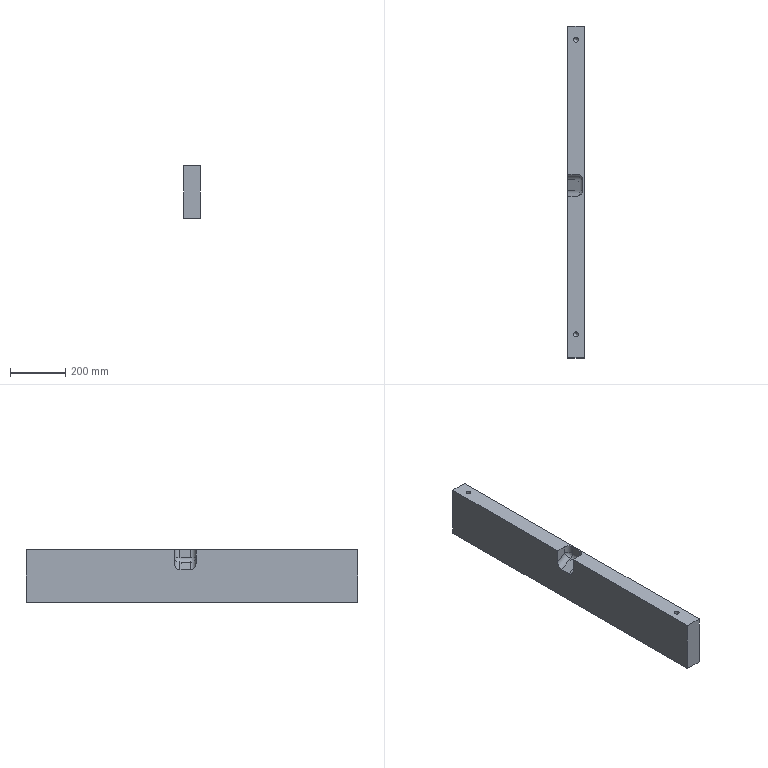Part | STEP file | lll_id4466_x_t | 1 solid | 26 faces | box 60 x 1200 x 190 mm | volume 13409835 mm3 | plane 10 | cylinder 9 | cone 5 | sphere 2 | commonest cylinder face diameters 40 x5 17.505 x2 17.506 x2
STEP:
#1=CARTESIAN_POINT('',(1461.188,550.,-370.));
#2=VERTEX_POINT('',#1);
#3=CARTESIAN_POINT('',(1452.435,550.,-370.));
#4=DIRECTION('',(0.,0.,1.));
#5=DIRECTION('',(1.,0.,0.));
#6=AXIS2_PLACEMENT_3D('',#3,#4,#5);
#7=CIRCLE('',#6,8.752);
#8=EDGE_CURVE('',#2,#2,#7,.T.);
#9=ORIENTED_EDGE('',*,*,#8,.T.);
#10=EDGE_LOOP('',(#9));
#11=FACE_BOUND('',#10,.T.);
#12=CARTESIAN_POINT('',(1422.435,600.,-370.));
#13=VERTEX_POINT('',#12);
#14=CARTESIAN_POINT('',(1422.435,-600.,-370.));
#15=VERTEX_POINT('',#14);
#16=CARTESIAN_POINT('',(1422.435,1.,-370.));
#17=DIRECTION('',(0.,-1.,0.));
#18=VECTOR('',#17,1.);
#19=LINE('',#16,#18);
#20=EDGE_CURVE('',#13,#15,#19,.T.);
#21=ORIENTED_EDGE('',*,*,#20,.F.);
#22=CARTESIAN_POINT('',(1482.435,600.,-370.));
#23=VERTEX_POINT('',#22);
#24=CARTESIAN_POINT('',(-2487.565,600.,-370.));
#25=DIRECTION('',(1.,0.,0.));
#26=VECTOR('',#25,1.);
#27=LINE('',#24,#26);
#28=EDGE_CURVE('',#13,#23,#27,.T.);
#29=ORIENTED_EDGE('',*,*,#28,.T.);
#30=CARTESIAN_POINT('',(1482.435,-600.,-370.));
#31=VERTEX_POINT('',#30);
#32=CARTESIAN_POINT('',(1482.435,600.,-370.));
#33=DIRECTION('',(0.,-1.,0.));
#34=VECTOR('',#33,1.);
#35=LINE('',#32,#34);
#36=EDGE_CURVE('',#23,#31,#35,.T.);
#37=ORIENTED_EDGE('',*,*,#36,.T.);
#38=CARTESIAN_POINT('',(1482.435,-600.,-370.));
#39=DIRECTION('',(-1.,0.,0.));
#40=VECTOR('',#39,1.);
#41=LINE('',#38,#40);
#42=EDGE_CURVE('',#31,#15,#41,.T.);
#43=ORIENTED_EDGE('',*,*,#42,.T.);
#44=EDGE_LOOP('',(#21,#29,#37,#43));
#45=FACE_BOUND('',#44,.T.);
#46=CARTESIAN_POINT('',(1461.188,-515.,-370.));
#47=VERTEX_POINT('',#46);
#48=CARTESIAN_POINT('',(1452.435,-515.,-370.));
#49=DIRECTION('',(0.,0.,1.));
#50=DIRECTION('',(1.,0.,0.));
#51=AXIS2_PLACEMENT_3D('',#48,#49,#50);
#52=CIRCLE('',#51,8.752);
#53=EDGE_CURVE('',#47,#47,#52,.T.);
#54=ORIENTED_EDGE('',*,*,#53,.T.);
#55=EDGE_LOOP('',(#54));
#56=FACE_BOUND('',#55,.T.);
#57=CARTESIAN_POINT('',(3668.751,1.,-370.));
#58=DIRECTION('',(0.,0.,-1.));
#59=DIRECTION('',(-1.,0.,0.));
#60=AXIS2_PLACEMENT_3D('',#57,#58,#59);
#61=PLANE('',#60);
#62=ADVANCED_FACE('',(#11,#45,#56),#61,.T.);
#63=CARTESIAN_POINT('',(1422.435,-15.,-180.));
#64=VERTEX_POINT('',#63);
#65=CARTESIAN_POINT('',(1422.435,-15.,-229.633));
#66=VERTEX_POINT('',#65);
#67=CARTESIAN_POINT('',(1422.435,-15.,-251.25));
#68=DIRECTION('',(0.,0.,-1.));
#69=VECTOR('',#68,1.);
#70=LINE('',#67,#69);
#71=EDGE_CURVE('',#64,#66,#70,.T.);
#72=ORIENTED_EDGE('',*,*,#71,.T.);
#73=CARTESIAN_POINT('',(1422.435,5.,-252.727));
#74=VERTEX_POINT('',#73);
#75=CARTESIAN_POINT('',(1422.435,5.,-229.633));
#76=DIRECTION('',(1.,0.,0.));
#77=DIRECTION('',(0.,0.,1.));
#78=AXIS2_PLACEMENT_3D('',#75,#76,#77);
#79=ELLIPSE('',#78,23.094,20.);
#80=EDGE_CURVE('',#66,#74,#79,.T.);
#81=ORIENTED_EDGE('',*,*,#80,.T.);
#82=CARTESIAN_POINT('',(1422.435,43.5,-252.727));
#83=VERTEX_POINT('',#82);
#84=CARTESIAN_POINT('',(1422.435,0.,-252.727));
#85=DIRECTION('',(0.,1.,0.));
#86=VECTOR('',#85,1.);
#87=LINE('',#84,#86);
#88=EDGE_CURVE('',#74,#83,#87,.T.);
#89=ORIENTED_EDGE('',*,*,#88,.T.);
#90=CARTESIAN_POINT('',(1422.435,63.5,-229.633));
#91=VERTEX_POINT('',#90);
#92=CARTESIAN_POINT('',(1422.435,43.5,-229.633));
#93=DIRECTION('',(1.,0.,0.));
#94=DIRECTION('',(0.,0.,-1.));
#95=AXIS2_PLACEMENT_3D('',#92,#93,#94);
#96=ELLIPSE('',#95,23.094,20.);
#97=EDGE_CURVE('',#83,#91,#96,.T.);
#98=ORIENTED_EDGE('',*,*,#97,.T.);
#99=CARTESIAN_POINT('',(1422.435,63.5,-180.));
#100=VERTEX_POINT('',#99);
#101=CARTESIAN_POINT('',(1422.435,63.5,-251.25));
#102=DIRECTION('',(0.,0.,1.));
#103=VECTOR('',#102,1.);
#104=LINE('',#101,#103);
#105=EDGE_CURVE('',#91,#100,#104,.T.);
#106=ORIENTED_EDGE('',*,*,#105,.T.);
#107=CARTESIAN_POINT('',(1422.435,600.,-180.));
#108=VERTEX_POINT('',#107);
#109=CARTESIAN_POINT('',(1422.435,0.,-180.));
#110=DIRECTION('',(0.,1.,0.));
#111=VECTOR('',#110,1.);
#112=LINE('',#109,#111);
#113=EDGE_CURVE('',#100,#108,#112,.T.);
#114=ORIENTED_EDGE('',*,*,#113,.T.);
#115=CARTESIAN_POINT('',(1422.435,600.,-182.5));
#116=DIRECTION('',(0.,0.,1.));
#117=VECTOR('',#116,1.);
#118=LINE('',#115,#117);
#119=EDGE_CURVE('',#13,#108,#118,.T.);
#120=ORIENTED_EDGE('',*,*,#119,.F.);
#121=ORIENTED_EDGE('',*,*,#20,.T.);
#122=CARTESIAN_POINT('',(1422.435,-600.,-180.));
#123=VERTEX_POINT('',#122);
#124=CARTESIAN_POINT('',(1422.435,-600.,-182.5));
#125=DIRECTION('',(0.,0.,-1.));
#126=VECTOR('',#125,1.);
#127=LINE('',#124,#126);
#128=EDGE_CURVE('',#123,#15,#127,.T.);
#129=ORIENTED_EDGE('',*,*,#128,.F.);
#130=CARTESIAN_POINT('',(1422.435,0.,-180.));
#131=DIRECTION('',(0.,1.,0.));
#132=VECTOR('',#131,1.);
#133=LINE('',#130,#132);
#134=EDGE_CURVE('',#123,#64,#133,.T.);
#135=ORIENTED_EDGE('',*,*,#134,.T.);
#136=EDGE_LOOP('',(#72,#81,#89,#98,#106,#114,#120,#121,#129,#135));
#137=FACE_OUTER_BOUND('',#136,.T.);
#138=CARTESIAN_POINT('',(1422.435,0.,-251.25));
#139=DIRECTION('',(1.,0.,0.));
#140=DIRECTION('',(0.,0.,-1.));
#141=AXIS2_PLACEMENT_3D('',#138,#139,#140);
#142=PLANE('',#141);
#143=ADVANCED_FACE('',(#137),#142,.F.);
#144=ORIENTED_EDGE('',*,*,#36,.F.);
#145=CARTESIAN_POINT('',(1482.435,600.,-180.));
#146=VERTEX_POINT('',#145);
#147=CARTESIAN_POINT('',(1482.435,600.,-182.5));
#148=DIRECTION('',(0.,0.,-1.));
#149=VECTOR('',#148,1.);
#150=LINE('',#147,#149);
#151=EDGE_CURVE('',#146,#23,#150,.T.);
#152=ORIENTED_EDGE('',*,*,#151,.F.);
#153=CARTESIAN_POINT('',(1482.435,-600.,-180.));
#154=VERTEX_POINT('',#153);
#155=CARTESIAN_POINT('',(1482.435,1.,-180.));
#156=DIRECTION('',(0.,-1.,0.));
#157=VECTOR('',#156,1.);
#158=LINE('',#155,#157);
#159=EDGE_CURVE('',#146,#154,#158,.T.);
#160=ORIENTED_EDGE('',*,*,#159,.T.);
#161=CARTESIAN_POINT('',(1482.435,-600.,-182.5));
#162=DIRECTION('',(0.,0.,-1.));
#163=VECTOR('',#162,1.);
#164=LINE('',#161,#163);
#165=EDGE_CURVE('',#154,#31,#164,.T.);
#166=ORIENTED_EDGE('',*,*,#165,.T.);
#167=EDGE_LOOP('',(#144,#152,#160,#166));
#168=FACE_OUTER_BOUND('',#167,.T.);
#169=CARTESIAN_POINT('',(1482.435,600.,-182.5));
#170=DIRECTION('',(1.,0.,0.));
#171=DIRECTION('',(0.,0.,-1.));
#172=AXIS2_PLACEMENT_3D('',#169,#170,#171);
#173=PLANE('',#172);
#174=ADVANCED_FACE('',(#168),#173,.T.);
#175=ORIENTED_EDGE('',*,*,#128,.T.);
#176=ORIENTED_EDGE('',*,*,#42,.F.);
#177=ORIENTED_EDGE('',*,*,#165,.F.);
#178=CARTESIAN_POINT('',(3668.751,-600.,-180.));
#179=DIRECTION('',(-1.,0.,0.));
#180=VECTOR('',#179,1.);
#181=LINE('',#178,#180);
#182=EDGE_CURVE('',#154,#123,#181,.T.);
#183=ORIENTED_EDGE('',*,*,#182,.T.);
#184=EDGE_LOOP('',(#175,#176,#177,#183));
#185=FACE_OUTER_BOUND('',#184,.T.);
#186=CARTESIAN_POINT('',(1482.435,-600.,-182.5));
#187=DIRECTION('',(0.,-1.,0.));
#188=DIRECTION('',(0.,0.,-1.));
#189=AXIS2_PLACEMENT_3D('',#186,#187,#188);
#190=PLANE('',#189);
#191=ADVANCED_FACE('',(#185),#190,.T.);
#192=ORIENTED_EDGE('',*,*,#119,.T.);
#193=CARTESIAN_POINT('',(3668.751,600.,-180.));
#194=DIRECTION('',(1.,0.,0.));
#195=VECTOR('',#194,1.);
#196=LINE('',#193,#195);
#197=EDGE_CURVE('',#108,#146,#196,.T.);
#198=ORIENTED_EDGE('',*,*,#197,.T.);
#199=ORIENTED_EDGE('',*,*,#151,.T.);
#200=ORIENTED_EDGE('',*,*,#28,.F.);
#201=EDGE_LOOP('',(#192,#198,#199,#200));
#202=FACE_OUTER_BOUND('',#201,.T.);
#203=CARTESIAN_POINT('',(-2487.565,600.,-182.5));
#204=DIRECTION('',(0.,1.,0.));
#205=DIRECTION('',(0.,0.,1.));
#206=AXIS2_PLACEMENT_3D('',#203,#204,#205);
#207=PLANE('',#206);
#208=ADVANCED_FACE('',(#202),#207,.T.);
#209=CARTESIAN_POINT('',(1443.682,550.,-180.));
#210=VERTEX_POINT('',#209);
#211=CARTESIAN_POINT('',(1452.435,550.,-180.));
#212=DIRECTION('',(0.,0.,-1.));
#213=DIRECTION('',(-1.,0.,0.));
#214=AXIS2_PLACEMENT_3D('',#211,#212,#213);
#215=CIRCLE('',#214,8.753);
#216=EDGE_CURVE('',#210,#210,#215,.T.);
#217=ORIENTED_EDGE('',*,*,#216,.T.);
#218=EDGE_LOOP('',(#217));
#219=FACE_BOUND('',#218,.T.);
#220=CARTESIAN_POINT('',(1443.682,-515.,-180.));
#221=VERTEX_POINT('',#220);
#222=CARTESIAN_POINT('',(1452.435,-515.,-180.));
#223=DIRECTION('',(0.,0.,-1.));
#224=DIRECTION('',(-1.,0.,0.));
#225=AXIS2_PLACEMENT_3D('',#222,#223,#224);
#226=CIRCLE('',#225,8.753);
#227=EDGE_CURVE('',#221,#221,#226,.T.);
#228=ORIENTED_EDGE('',*,*,#227,.T.);
#229=EDGE_LOOP('',(#228));
#230=FACE_BOUND('',#229,.T.);
#231=CARTESIAN_POINT('',(1457.5,63.5,-180.));
#232=VERTEX_POINT('',#231);
#233=CARTESIAN_POINT('',(3668.751,63.5,-180.));
#234=DIRECTION('',(1.,0.,0.));
#235=VECTOR('',#234,1.);
#236=LINE('',#233,#235);
#237=EDGE_CURVE('',#100,#232,#236,.T.);
#238=ORIENTED_EDGE('',*,*,#237,.T.);
#239=CARTESIAN_POINT('',(1477.5,43.5,-180.));
#240=VERTEX_POINT('',#239);
#241=CARTESIAN_POINT('',(1457.5,43.5,-180.));
#242=DIRECTION('',(0.,0.,-1.));
#243=DIRECTION('',(-1.,0.,0.));
#244=AXIS2_PLACEMENT_3D('',#241,#242,#243);
#245=CIRCLE('',#244,20.);
#246=EDGE_CURVE('',#232,#240,#245,.T.);
#247=ORIENTED_EDGE('',*,*,#246,.T.);
#248=CARTESIAN_POINT('',(1477.5,5.,-180.));
#249=VERTEX_POINT('',#248);
#250=CARTESIAN_POINT('',(1477.5,1.,-180.));
#251=DIRECTION('',(0.,-1.,0.));
#252=VECTOR('',#251,1.);
#253=LINE('',#250,#252);
#254=EDGE_CURVE('',#240,#249,#253,.T.);
#255=ORIENTED_EDGE('',*,*,#254,.T.);
#256=CARTESIAN_POINT('',(1457.5,-15.,-180.));
#257=VERTEX_POINT('',#256);
#258=CARTESIAN_POINT('',(1457.5,5.,-180.));
#259=DIRECTION('',(0.,0.,-1.));
#260=DIRECTION('',(-1.,0.,0.));
#261=AXIS2_PLACEMENT_3D('',#258,#259,#260);
#262=CIRCLE('',#261,20.);
#263=EDGE_CURVE('',#249,#257,#262,.T.);
#264=ORIENTED_EDGE('',*,*,#263,.T.);
#265=CARTESIAN_POINT('',(3668.751,-15.,-180.));
#266=DIRECTION('',(-1.,0.,0.));
#267=VECTOR('',#266,1.);
#268=LINE('',#265,#267);
#269=EDGE_CURVE('',#257,#64,#268,.T.);
#270=ORIENTED_EDGE('',*,*,#269,.T.);
#271=ORIENTED_EDGE('',*,*,#134,.F.);
#272=ORIENTED_EDGE('',*,*,#182,.F.);
#273=ORIENTED_EDGE('',*,*,#159,.F.);
#274=ORIENTED_EDGE('',*,*,#197,.F.);
#275=ORIENTED_EDGE('',*,*,#113,.F.);
#276=EDGE_LOOP('',(#238,#247,#255,#264,#270,#271,#272,#273,#274,#275));
#277=FACE_BOUND('',#276,.T.);
#278=CARTESIAN_POINT('',(3668.751,1.,-180.));
#279=DIRECTION('',(0.,0.,-1.));
#280=DIRECTION('',(-1.,0.,0.));
#281=AXIS2_PLACEMENT_3D('',#278,#279,#280);
#282=PLANE('',#281);
#283=ADVANCED_FACE('',(#219,#230,#277),#282,.F.);
#284=CARTESIAN_POINT('',(1457.5,-15.,-209.388));
#285=VERTEX_POINT('',#284);
#286=CARTESIAN_POINT('',(1457.5,-15.,-205.));
#287=DIRECTION('',(0.,0.,-1.));
#288=VECTOR('',#287,1.);
#289=LINE('',#286,#288);
#290=EDGE_CURVE('',#257,#285,#289,.T.);
#291=ORIENTED_EDGE('',*,*,#290,.T.);
#292=CARTESIAN_POINT('',(1446.251,-15.,-215.883));
#293=DIRECTION('',(-0.866,0.,-0.5));
#294=VECTOR('',#293,1.);
#295=LINE('',#292,#294);
#296=EDGE_CURVE('',#285,#66,#295,.T.);
#297=ORIENTED_EDGE('',*,*,#296,.T.);
#298=ORIENTED_EDGE('',*,*,#71,.F.);
#299=ORIENTED_EDGE('',*,*,#269,.F.);
#300=EDGE_LOOP('',(#291,#297,#298,#299));
#301=FACE_OUTER_BOUND('',#300,.T.);
#302=CARTESIAN_POINT('',(1439.968,-15.,-205.));
#303=DIRECTION('',(0.,-1.,0.));
#304=DIRECTION('',(0.,0.,-1.));
#305=AXIS2_PLACEMENT_3D('',#302,#303,#304);
#306=PLANE('',#305);
#307=ADVANCED_FACE('',(#301),#306,.F.);
#308=CARTESIAN_POINT('',(1457.5,63.5,-209.388));
#309=VERTEX_POINT('',#308);
#310=CARTESIAN_POINT('',(1446.251,63.5,-215.883));
#311=DIRECTION('',(0.866,0.,0.5));
#312=VECTOR('',#311,1.);
#313=LINE('',#310,#312);
#314=EDGE_CURVE('',#91,#309,#313,.T.);
#315=ORIENTED_EDGE('',*,*,#314,.T.);
#316=CARTESIAN_POINT('',(1457.5,63.5,-205.));
#317=DIRECTION('',(0.,0.,-1.));
#318=VECTOR('',#317,1.);
#319=LINE('',#316,#318);
#320=EDGE_CURVE('',#232,#309,#319,.T.);
#321=ORIENTED_EDGE('',*,*,#320,.F.);
#322=ORIENTED_EDGE('',*,*,#237,.F.);
#323=ORIENTED_EDGE('',*,*,#105,.F.);
#324=EDGE_LOOP('',(#315,#321,#322,#323));
#325=FACE_OUTER_BOUND('',#324,.T.);
#326=CARTESIAN_POINT('',(1439.968,63.5,-205.));
#327=DIRECTION('',(0.,1.,0.));
#328=DIRECTION('',(0.,0.,1.));
#329=AXIS2_PLACEMENT_3D('',#326,#327,#328);
#330=PLANE('',#329);
#331=ADVANCED_FACE('',(#325),#330,.F.);
#332=CARTESIAN_POINT('',(1477.5,43.5,-209.388));
#333=VERTEX_POINT('',#332);
#334=CARTESIAN_POINT('',(1477.5,43.5,-205.));
#335=DIRECTION('',(0.,0.,-1.));
#336=VECTOR('',#335,1.);
#337=LINE('',#334,#336);
#338=EDGE_CURVE('',#240,#333,#337,.T.);
#339=ORIENTED_EDGE('',*,*,#338,.T.);
#340=CARTESIAN_POINT('',(1477.5,5.,-209.388));
#341=VERTEX_POINT('',#340);
#342=CARTESIAN_POINT('',(1477.5,24.25,-209.388));
#343=DIRECTION('',(0.,-1.,0.));
#344=VECTOR('',#343,1.);
#345=LINE('',#342,#344);
#346=EDGE_CURVE('',#333,#341,#345,.T.);
#347=ORIENTED_EDGE('',*,*,#346,.T.);
#348=CARTESIAN_POINT('',(1477.5,5.,-205.));
#349=DIRECTION('',(0.,0.,1.));
#350=VECTOR('',#349,1.);
#351=LINE('',#348,#350);
#352=EDGE_CURVE('',#341,#249,#351,.T.);
#353=ORIENTED_EDGE('',*,*,#352,.T.);
#354=ORIENTED_EDGE('',*,*,#254,.F.);
#355=EDGE_LOOP('',(#339,#347,#353,#354));
#356=FACE_OUTER_BOUND('',#355,.T.);
#357=CARTESIAN_POINT('',(1477.5,24.25,-205.));
#358=DIRECTION('',(1.,0.,0.));
#359=DIRECTION('',(0.,0.,-1.));
#360=AXIS2_PLACEMENT_3D('',#357,#358,#359);
#361=PLANE('',#360);
#362=ADVANCED_FACE('',(#356),#361,.F.);
#363=ORIENTED_EDGE('',*,*,#352,.F.);
#364=CARTESIAN_POINT('',(1457.5,5.,-209.388));
#365=DIRECTION('',(0.,0.,-1.));
#366=DIRECTION('',(-1.,0.,0.));
#367=AXIS2_PLACEMENT_3D('',#364,#365,#366);
#368=CIRCLE('',#367,20.);
#369=EDGE_CURVE('',#341,#285,#368,.T.);
#370=ORIENTED_EDGE('',*,*,#369,.T.);
#371=ORIENTED_EDGE('',*,*,#290,.F.);
#372=ORIENTED_EDGE('',*,*,#263,.F.);
#373=EDGE_LOOP('',(#363,#370,#371,#372));
#374=FACE_OUTER_BOUND('',#373,.T.);
#375=CARTESIAN_POINT('',(1457.5,5.,-205.));
#376=DIRECTION('',(0.,0.,-1.));
#377=DIRECTION('',(-1.,0.,0.));
#378=AXIS2_PLACEMENT_3D('',#375,#376,#377);
#379=CYLINDRICAL_SURFACE('',#378,20.);
#380=ADVANCED_FACE('',(#374),#379,.F.);
#381=ORIENTED_EDGE('',*,*,#246,.F.);
#382=ORIENTED_EDGE('',*,*,#320,.T.);
#383=CARTESIAN_POINT('',(1457.5,43.5,-209.388));
#384=DIRECTION('',(0.,0.,-1.));
#385=DIRECTION('',(-1.,0.,0.));
#386=AXIS2_PLACEMENT_3D('',#383,#384,#385);
#387=CIRCLE('',#386,20.);
#388=EDGE_CURVE('',#309,#333,#387,.T.);
#389=ORIENTED_EDGE('',*,*,#388,.T.);
#390=ORIENTED_EDGE('',*,*,#338,.F.);
#391=EDGE_LOOP('',(#381,#382,#389,#390));
#392=FACE_OUTER_BOUND('',#391,.T.);
#393=CARTESIAN_POINT('',(1457.5,43.5,-205.));
#394=DIRECTION('',(0.,0.,-1.));
#395=DIRECTION('',(-1.,0.,0.));
#396=AXIS2_PLACEMENT_3D('',#393,#394,#395);
#397=CYLINDRICAL_SURFACE('',#396,20.);
#398=ADVANCED_FACE('',(#392),#397,.F.);
#399=CARTESIAN_POINT('',(1462.288,38.,-229.718));
#400=VERTEX_POINT('',#399);
#401=CARTESIAN_POINT('',(1462.106,38.,-229.823));
#402=DIRECTION('',(0.5,0.,-0.866));
#403=DIRECTION('',(0.866,0.,0.5));
#404=AXIS2_PLACEMENT_3D('',#401,#402,#403);
#405=ELLIPSE('',#404,0.211,0.1492);
#406=EDGE_CURVE('',#400,#400,#405,.T.);
#407=ORIENTED_EDGE('',*,*,#406,.T.);
#408=EDGE_LOOP('',(#407));
#409=FACE_BOUND('',#408,.T.);
#410=ORIENTED_EDGE('',*,*,#88,.F.);
#411=CARTESIAN_POINT('',(1467.5,5.,-226.709));
#412=VERTEX_POINT('',#411);
#413=CARTESIAN_POINT('',(1410.06,5.,-259.872));
#414=DIRECTION('',(0.866,0.,0.5));
#415=VECTOR('',#414,1.);
#416=LINE('',#413,#415);
#417=EDGE_CURVE('',#74,#412,#416,.T.);
#418=ORIENTED_EDGE('',*,*,#417,.T.);
#419=CARTESIAN_POINT('',(1467.5,43.5,-226.709));
#420=VERTEX_POINT('',#419);
#421=CARTESIAN_POINT('',(1467.5,0.,-226.709));
#422=DIRECTION('',(0.,1.,0.));
#423=VECTOR('',#422,1.);
#424=LINE('',#421,#423);
#425=EDGE_CURVE('',#412,#420,#424,.T.);
#426=ORIENTED_EDGE('',*,*,#425,.T.);
#427=CARTESIAN_POINT('',(1410.06,43.5,-259.872));
#428=DIRECTION('',(-0.866,0.,-0.5));
#429=VECTOR('',#428,1.);
#430=LINE('',#427,#429);
#431=EDGE_CURVE('',#420,#83,#430,.T.);
#432=ORIENTED_EDGE('',*,*,#431,.T.);
#433=EDGE_LOOP('',(#410,#418,#426,#432));
#434=FACE_BOUND('',#433,.T.);
#435=CARTESIAN_POINT('',(1410.06,0.,-259.872));
#436=DIRECTION('',(0.5,0.,-0.866));
#437=DIRECTION('',(0.,1.,0.));
#438=AXIS2_PLACEMENT_3D('',#435,#436,#437);
#439=PLANE('',#438);
#440=ADVANCED_FACE('',(#409,#434),#439,.F.);
#441=CARTESIAN_POINT('',(1457.5,43.5,-209.388));
#442=DIRECTION('',(-0.866,0.,-0.5));
#443=DIRECTION('',(-0.5,0.,0.866));
#444=AXIS2_PLACEMENT_3D('',#441,#442,#443);
#445=CIRCLE('',#444,20.);
#446=EDGE_CURVE('',#309,#420,#445,.T.);
#447=ORIENTED_EDGE('',*,*,#446,.F.);
#448=ORIENTED_EDGE('',*,*,#314,.F.);
#449=ORIENTED_EDGE('',*,*,#97,.F.);
#450=ORIENTED_EDGE('',*,*,#431,.F.);
#451=EDGE_LOOP('',(#447,#448,#449,#450));
#452=FACE_OUTER_BOUND('',#451,.T.);
#453=CARTESIAN_POINT('',(1446.251,43.5,-215.883));
#454=DIRECTION('',(-0.866,0.,-0.5));
#455=DIRECTION('',(-0.5,0.,0.866));
#456=AXIS2_PLACEMENT_3D('',#453,#454,#455);
#457=CYLINDRICAL_SURFACE('',#456,20.);
#458=ADVANCED_FACE('',(#452),#457,.F.);
#459=ORIENTED_EDGE('',*,*,#388,.F.);
#460=ORIENTED_EDGE('',*,*,#446,.T.);
#461=CARTESIAN_POINT('',(1457.5,43.5,-209.388));
#462=DIRECTION('',(0.,1.,0.));
#463=DIRECTION('',(0.,0.,1.));
#464=AXIS2_PLACEMENT_3D('',#461,#462,#463);
#465=CIRCLE('',#464,20.);
#466=EDGE_CURVE('',#333,#420,#465,.T.);
#467=ORIENTED_EDGE('',*,*,#466,.F.);
#468=EDGE_LOOP('',(#459,#460,#467));
#469=FACE_OUTER_BOUND('',#468,.T.);
#470=CARTESIAN_POINT('',(1457.5,43.5,-209.388));
#471=DIRECTION('',(0.,0.,1.));
#472=DIRECTION('',(1.,0.,0.));
#473=AXIS2_PLACEMENT_3D('',#470,#471,#472);
#474=SPHERICAL_SURFACE('',#473,20.);
#475=ADVANCED_FACE('',(#469),#474,.F.);
#476=CARTESIAN_POINT('',(1457.5,5.,-209.388));
#477=DIRECTION('',(0.,1.,0.));
#478=DIRECTION('',(0.,0.,1.));
#479=AXIS2_PLACEMENT_3D('',#476,#477,#478);
#480=CIRCLE('',#479,20.);
#481=EDGE_CURVE('',#341,#412,#480,.T.);
#482=ORIENTED_EDGE('',*,*,#481,.F.);
#483=ORIENTED_EDGE('',*,*,#346,.F.);
#484=ORIENTED_EDGE('',*,*,#466,.T.);
#485=ORIENTED_EDGE('',*,*,#425,.F.);
#486=EDGE_LOOP('',(#482,#483,#484,#485));
#487=FACE_OUTER_BOUND('',#486,.T.);
#488=CARTESIAN_POINT('',(1457.5,24.25,-209.388));
#489=DIRECTION('',(0.,1.,0.));
#490=DIRECTION('',(0.,0.,1.));
#491=AXIS2_PLACEMENT_3D('',#488,#489,#490);
#492=CYLINDRICAL_SURFACE('',#491,20.);
#493=ADVANCED_FACE('',(#487),#492,.F.);
#494=ORIENTED_EDGE('',*,*,#369,.F.);
#495=ORIENTED_EDGE('',*,*,#481,.T.);
#496=CARTESIAN_POINT('',(1457.5,5.,-209.388));
#497=DIRECTION('',(0.866,0.,0.5));
#498=DIRECTION('',(0.5,0.,-0.866));
#499=AXIS2_PLACEMENT_3D('',#496,#497,#498);
#500=CIRCLE('',#499,20.);
#501=EDGE_CURVE('',#285,#412,#500,.T.);
#502=ORIENTED_EDGE('',*,*,#501,.F.);
#503=EDGE_LOOP('',(#494,#495,#502));
#504=FACE_OUTER_BOUND('',#503,.T.);
#505=CARTESIAN_POINT('',(1457.5,5.,-209.388));
#506=DIRECTION('',(0.,0.,1.));
#507=DIRECTION('',(1.,0.,0.));
#508=AXIS2_PLACEMENT_3D('',#505,#506,#507);
#509=SPHERICAL_SURFACE('',#508,20.);
#510=ADVANCED_FACE('',(#504),#509,.F.);
#511=ORIENTED_EDGE('',*,*,#501,.T.);
#512=ORIENTED_EDGE('',*,*,#417,.F.);
#513=ORIENTED_EDGE('',*,*,#80,.F.);
#514=ORIENTED_EDGE('',*,*,#296,.F.);
#515=EDGE_LOOP('',(#511,#512,#513,#514));
#516=FACE_OUTER_BOUND('',#515,.T.);
#517=CARTESIAN_POINT('',(1446.251,5.,-215.883));
#518=DIRECTION('',(0.866,0.,0.5));
#519=DIRECTION('',(0.5,0.,-0.866));
#520=AXIS2_PLACEMENT_3D('',#517,#518,#519);
#521=CYLINDRICAL_SURFACE('',#520,20.);
#522=ADVANCED_FACE('',(#516),#521,.F.);
#523=CARTESIAN_POINT('',(1461.188,550.,-328.747));
#524=VERTEX_POINT('',#523);
#525=CARTESIAN_POINT('',(1452.435,550.,-328.747));
#526=DIRECTION('',(0.,0.,1.));
#527=DIRECTION('',(1.,0.,0.));
#528=AXIS2_PLACEMENT_3D('',#525,#526,#527);
#529=CIRCLE('',#528,8.752);
#530=EDGE_CURVE('',#524,#524,#529,.T.);
#531=ORIENTED_EDGE('',*,*,#530,.T.);
#532=EDGE_LOOP('',(#531));
#533=FACE_BOUND('',#532,.T.);
#534=ORIENTED_EDGE('',*,*,#8,.F.);
#535=EDGE_LOOP('',(#534));
#536=FACE_BOUND('',#535,.T.);
#537=CARTESIAN_POINT('',(1452.435,550.,-370.));
#538=DIRECTION('',(0.,0.,1.));
#539=DIRECTION('',(-1.,0.,0.));
#540=AXIS2_PLACEMENT_3D('',#537,#538,#539);
#541=CYLINDRICAL_SURFACE('',#540,8.752);
#542=ADVANCED_FACE('',(#533,#536),#541,.F.);
#543=CARTESIAN_POINT('',(1452.435,550.,-319.994));
#544=VERTEX_POINT('',#543);
#545=VERTEX_LOOP('',#544);
#546=FACE_BOUND('',#545,.T.);
#547=ORIENTED_EDGE('',*,*,#530,.F.);
#548=EDGE_LOOP('',(#547));
#549=FACE_BOUND('',#548,.T.);
#550=CARTESIAN_POINT('',(1452.435,550.,-328.747));
#551=DIRECTION('',(0.,0.,-1.));
#552=DIRECTION('',(1.,0.,0.));
#553=AXIS2_PLACEMENT_3D('',#550,#551,#552);
#554=CONICAL_SURFACE('',#553,8.752,45.);
#555=ADVANCED_FACE('',(#546,#549),#554,.F.);
#556=CARTESIAN_POINT('',(1461.188,-515.,-328.747));
#557=VERTEX_POINT('',#556);
#558=CARTESIAN_POINT('',(1452.435,-515.,-328.747));
#559=DIRECTION('',(0.,0.,1.));
#560=DIRECTION('',(1.,0.,0.));
#561=AXIS2_PLACEMENT_3D('',#558,#559,#560);
#562=CIRCLE('',#561,8.752);
#563=EDGE_CURVE('',#557,#557,#562,.T.);
#564=ORIENTED_EDGE('',*,*,#563,.T.);
#565=EDGE_LOOP('',(#564));
#566=FACE_BOUND('',#565,.T.);
#567=ORIENTED_EDGE('',*,*,#53,.F.);
#568=EDGE_LOOP('',(#567));
#569=FACE_BOUND('',#568,.T.);
#570=CARTESIAN_POINT('',(1452.435,-515.,-370.));
#571=DIRECTION('',(0.,0.,1.));
#572=DIRECTION('',(-1.,0.,0.));
#573=AXIS2_PLACEMENT_3D('',#570,#571,#572);
#574=CYLINDRICAL_SURFACE('',#573,8.752);
#575=ADVANCED_FACE('',(#566,#569),#574,.F.);
#576=CARTESIAN_POINT('',(1452.435,-515.,-319.994));
#577=VERTEX_POINT('',#576);
#578=VERTEX_LOOP('',#577);
#579=FACE_BOUND('',#578,.T.);
#580=ORIENTED_EDGE('',*,*,#563,.F.);
#581=EDGE_LOOP('',(#580));
#582=FACE_BOUND('',#581,.T.);
#583=CARTESIAN_POINT('',(1452.435,-515.,-328.747));
#584=DIRECTION('',(0.,0.,-1.));
#585=DIRECTION('',(1.,0.,0.));
#586=AXIS2_PLACEMENT_3D('',#583,#584,#585);
#587=CONICAL_SURFACE('',#586,8.752,45.);
#588=ADVANCED_FACE('',(#579,#582),#587,.F.);
#589=CARTESIAN_POINT('',(1443.682,-515.,-221.253));
#590=VERTEX_POINT('',#589);
#591=CARTESIAN_POINT('',(1452.435,-515.,-221.253));
#592=DIRECTION('',(0.,0.,-1.));
#593=DIRECTION('',(-1.,0.,0.));
#594=AXIS2_PLACEMENT_3D('',#591,#592,#593);
#595=CIRCLE('',#594,8.753);
#596=EDGE_CURVE('',#590,#590,#595,.T.);
#597=ORIENTED_EDGE('',*,*,#596,.T.);
#598=EDGE_LOOP('',(#597));
#599=FACE_BOUND('',#598,.T.);
#600=ORIENTED_EDGE('',*,*,#227,.F.);
#601=EDGE_LOOP('',(#600));
#602=FACE_BOUND('',#601,.T.);
#603=CARTESIAN_POINT('',(1452.435,-515.,-180.));
#604=DIRECTION('',(0.,0.,-1.));
#605=DIRECTION('',(1.,0.,0.));
#606=AXIS2_PLACEMENT_3D('',#603,#604,#605);
#607=CYLINDRICAL_SURFACE('',#606,8.753);
#608=ADVANCED_FACE('',(#599,#602),#607,.F.);
#609=CARTESIAN_POINT('',(1452.435,-515.,-230.006));
#610=VERTEX_POINT('',#609);
#611=VERTEX_LOOP('',#610);
#612=FACE_BOUND('',#611,.T.);
#613=ORIENTED_EDGE('',*,*,#596,.F.);
#614=EDGE_LOOP('',(#613));
#615=FACE_BOUND('',#614,.T.);
#616=CARTESIAN_POINT('',(1452.435,-515.,-221.253));
#617=DIRECTION('',(0.,0.,1.));
#618=DIRECTION('',(-1.,0.,0.));
#619=AXIS2_PLACEMENT_3D('',#616,#617,#618);
#620=CONICAL_SURFACE('',#619,8.753,45.);
#621=ADVANCED_FACE('',(#612,#615),#620,.F.);
#622=CARTESIAN_POINT('',(1443.682,550.,-221.253));
#623=VERTEX_POINT('',#622);
#624=CARTESIAN_POINT('',(1452.435,550.,-221.253));
#625=DIRECTION('',(0.,0.,-1.));
#626=DIRECTION('',(-1.,0.,0.));
#627=AXIS2_PLACEMENT_3D('',#624,#625,#626);
#628=CIRCLE('',#627,8.753);
#629=EDGE_CURVE('',#623,#623,#628,.T.);
#630=ORIENTED_EDGE('',*,*,#629,.T.);
#631=EDGE_LOOP('',(#630));
#632=FACE_BOUND('',#631,.T.);
#633=ORIENTED_EDGE('',*,*,#216,.F.);
#634=EDGE_LOOP('',(#633));
#635=FACE_BOUND('',#634,.T.);
#636=CARTESIAN_POINT('',(1452.435,550.,-180.));
#637=DIRECTION('',(0.,0.,-1.));
#638=DIRECTION('',(1.,0.,0.));
#639=AXIS2_PLACEMENT_3D('',#636,#637,#638);
#640=CYLINDRICAL_SURFACE('',#639,8.753);
#641=ADVANCED_FACE('',(#632,#635),#640,.F.);
#642=CARTESIAN_POINT('',(1452.435,550.,-230.006));
#643=VERTEX_POINT('',#642);
#644=VERTEX_LOOP('',#643);
#645=FACE_BOUND('',#644,.T.);
#646=ORIENTED_EDGE('',*,*,#629,.F.);
#647=EDGE_LOOP('',(#646));
#648=FACE_BOUND('',#647,.T.);
#649=CARTESIAN_POINT('',(1452.435,550.,-221.253));
#650=DIRECTION('',(0.,0.,1.));
#651=DIRECTION('',(-1.,0.,0.));
#652=AXIS2_PLACEMENT_3D('',#649,#650,#651);
#653=CONICAL_SURFACE('',#652,8.753,45.);
#654=ADVANCED_FACE('',(#645,#648),#653,.F.);
#655=CARTESIAN_POINT('',(1462.,38.,-230.006));
#656=VERTEX_POINT('',#655);
#657=VERTEX_LOOP('',#656);
#658=FACE_BOUND('',#657,.T.);
#659=ORIENTED_EDGE('',*,*,#406,.F.);
#660=EDGE_LOOP('',(#659));
#661=FACE_BOUND('',#660,.T.);
#662=CARTESIAN_POINT('',(1462.,38.,-221.253));
#663=DIRECTION('',(0.,0.,1.));
#664=DIRECTION('',(-1.,0.,0.));
#665=AXIS2_PLACEMENT_3D('',#662,#663,#664);
#666=CONICAL_SURFACE('',#665,8.753,45.);
#667=ADVANCED_FACE('',(#658,#661),#666,.F.);
#668=CLOSED_SHELL('',(#62,#143,#174,#191,#208,#283,#307,#331,#362,#380,#398,#440,#458,#475,#493,#510,#522,#542,#555,#575,#588,#608,#621,#641,#654,#667));
#669=MANIFOLD_SOLID_BREP('',#668);
#670=(LENGTH_UNIT()NAMED_UNIT(*)SI_UNIT(.MILLI.,.METRE.));
#671=UNCERTAINTY_MEASURE_WITH_UNIT(LENGTH_MEASURE(0.00002),#670,'','');
#672=(NAMED_UNIT(*)PLANE_ANGLE_UNIT()SI_UNIT($,.RADIAN.));
#673=PLANE_ANGLE_MEASURE_WITH_UNIT(PLANE_ANGLE_MEASURE(0.01745),#672);
#674=DIMENSIONAL_EXPONENTS(0.,0.,0.,0.,0.,0.,0.);
#675=(CONVERSION_BASED_UNIT('DEGREE',#673)NAMED_UNIT(#674)PLANE_ANGLE_UNIT());
#676=(NAMED_UNIT(*)SI_UNIT($,.STERADIAN.)SOLID_ANGLE_UNIT());
#677=(GEOMETRIC_REPRESENTATION_CONTEXT(3)GLOBAL_UNCERTAINTY_ASSIGNED_CONTEXT((#671))GLOBAL_UNIT_ASSIGNED_CONTEXT((#670,#675,#676))REPRESENTATION_CONTEXT('',''));
#678=ADVANCED_BREP_SHAPE_REPRESENTATION('',(#669),#677);